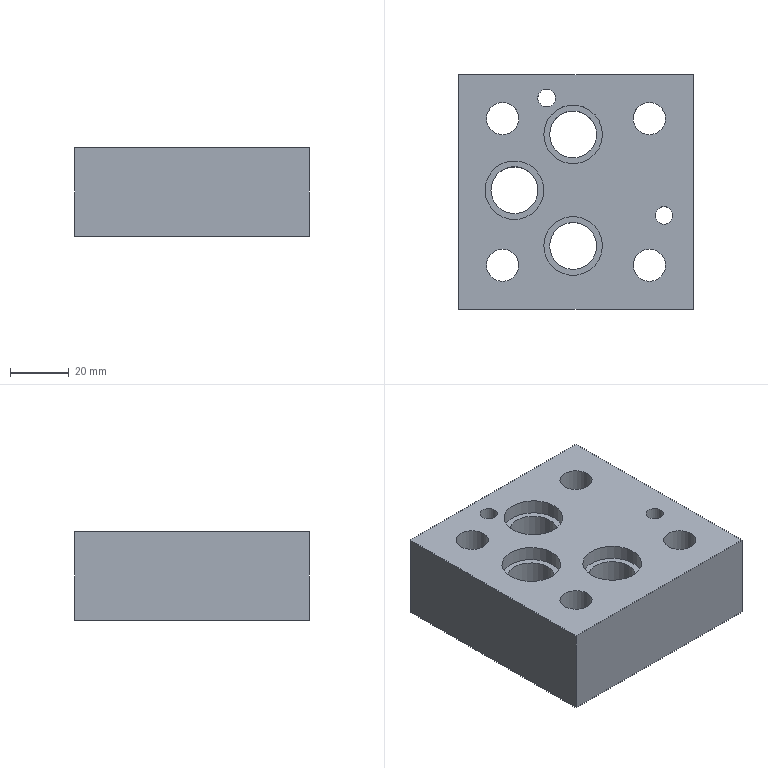Part | NX | features solid 2 | 1 solid | 29 faces | box 80 x 80 x 30 mm | volume 152774 mm3 | cylinder 16 | plane 13 | commonest cylinder face diameters 11 x4 17 x4 16 x3 20 x3 6 x2
STEP:
#1=CARTESIAN_POINT('',(-698.983,-4.404,58.));
#2=VERTEX_POINT('',#1);
#3=CARTESIAN_POINT('',(-690.983,-4.404,58.));
#4=DIRECTION('',(0.,0.,-1.));
#5=DIRECTION('',(-1.,0.,0.));
#6=AXIS2_PLACEMENT_3D('',#3,#4,#5);
#7=CIRCLE('',#6,8.);
#8=EDGE_CURVE('',#2,#2,#7,.F.);
#9=ORIENTED_EDGE('',*,*,#8,.T.);
#10=EDGE_LOOP('',(#9));
#11=FACE_BOUND('',#10,.T.);
#12=CARTESIAN_POINT('',(-703.5,-30.,58.));
#13=VERTEX_POINT('',#12);
#14=CARTESIAN_POINT('',(-695.,-30.,58.));
#15=DIRECTION('',(0.,0.,-1.));
#16=DIRECTION('',(-1.,0.,0.));
#17=AXIS2_PLACEMENT_3D('',#14,#15,#16);
#18=CIRCLE('',#17,8.5);
#19=EDGE_CURVE('',#13,#13,#18,.T.);
#20=ORIENTED_EDGE('',*,*,#19,.F.);
#21=EDGE_LOOP('',(#20));
#22=FACE_BOUND('',#21,.T.);
#23=CARTESIAN_POINT('',(-703.5,20.,58.));
#24=VERTEX_POINT('',#23);
#25=CARTESIAN_POINT('',(-695.,20.,58.));
#26=DIRECTION('',(0.,0.,-1.));
#27=DIRECTION('',(-1.,0.,0.));
#28=AXIS2_PLACEMENT_3D('',#25,#26,#27);
#29=CIRCLE('',#28,8.5);
#30=EDGE_CURVE('',#24,#24,#29,.T.);
#31=ORIENTED_EDGE('',*,*,#30,.F.);
#32=EDGE_LOOP('',(#31));
#33=FACE_BOUND('',#32,.T.);
#34=CARTESIAN_POINT('',(-653.5,20.,58.));
#35=VERTEX_POINT('',#34);
#36=CARTESIAN_POINT('',(-645.,20.,58.));
#37=DIRECTION('',(0.,0.,-1.));
#38=DIRECTION('',(-1.,0.,0.));
#39=AXIS2_PLACEMENT_3D('',#36,#37,#38);
#40=CIRCLE('',#39,8.5);
#41=EDGE_CURVE('',#35,#35,#40,.T.);
#42=ORIENTED_EDGE('',*,*,#41,.F.);
#43=EDGE_LOOP('',(#42));
#44=FACE_BOUND('',#43,.T.);
#45=CARTESIAN_POINT('',(-653.5,-30.,58.));
#46=VERTEX_POINT('',#45);
#47=CARTESIAN_POINT('',(-645.,-30.,58.));
#48=DIRECTION('',(0.,0.,-1.));
#49=DIRECTION('',(-1.,0.,0.));
#50=AXIS2_PLACEMENT_3D('',#47,#48,#49);
#51=CIRCLE('',#50,8.5);
#52=EDGE_CURVE('',#46,#46,#51,.T.);
#53=ORIENTED_EDGE('',*,*,#52,.F.);
#54=EDGE_LOOP('',(#53));
#55=FACE_BOUND('',#54,.T.);
#56=CARTESIAN_POINT('',(-710.,-45.,58.));
#57=VERTEX_POINT('',#56);
#58=CARTESIAN_POINT('',(-710.,35.,58.));
#59=VERTEX_POINT('',#58);
#60=CARTESIAN_POINT('',(-710.,25.,58.));
#61=DIRECTION('',(0.,1.,0.));
#62=VECTOR('',#61,1000.);
#63=LINE('',#60,#62);
#64=EDGE_CURVE('',#57,#59,#63,.T.);
#65=ORIENTED_EDGE('',*,*,#64,.T.);
#66=CARTESIAN_POINT('',(-630.,35.,58.));
#67=VERTEX_POINT('',#66);
#68=CARTESIAN_POINT('',(-720.,35.,58.));
#69=DIRECTION('',(1.,0.,0.));
#70=VECTOR('',#69,1000.);
#71=LINE('',#68,#70);
#72=EDGE_CURVE('',#59,#67,#71,.T.);
#73=ORIENTED_EDGE('',*,*,#72,.T.);
#74=CARTESIAN_POINT('',(-630.,-45.,58.));
#75=VERTEX_POINT('',#74);
#76=CARTESIAN_POINT('',(-630.,25.,58.));
#77=DIRECTION('',(0.,-1.,0.));
#78=VECTOR('',#77,1000.);
#79=LINE('',#76,#78);
#80=EDGE_CURVE('',#67,#75,#79,.T.);
#81=ORIENTED_EDGE('',*,*,#80,.T.);
#82=CARTESIAN_POINT('',(-720.,-45.,58.));
#83=DIRECTION('',(-1.,0.,0.));
#84=VECTOR('',#83,1000.);
#85=LINE('',#82,#84);
#86=EDGE_CURVE('',#75,#57,#85,.T.);
#87=ORIENTED_EDGE('',*,*,#86,.T.);
#88=EDGE_LOOP('',(#65,#73,#81,#87));
#89=FACE_BOUND('',#88,.T.);
#90=CARTESIAN_POINT('',(-678.983,14.595,58.));
#91=VERTEX_POINT('',#90);
#92=CARTESIAN_POINT('',(-670.983,14.595,58.));
#93=DIRECTION('',(0.,0.,-1.));
#94=DIRECTION('',(-1.,0.,0.));
#95=AXIS2_PLACEMENT_3D('',#92,#93,#94);
#96=CIRCLE('',#95,8.);
#97=EDGE_CURVE('',#91,#91,#96,.T.);
#98=ORIENTED_EDGE('',*,*,#97,.F.);
#99=EDGE_LOOP('',(#98));
#100=FACE_BOUND('',#99,.T.);
#101=CARTESIAN_POINT('',(-678.983,-23.404,58.));
#102=VERTEX_POINT('',#101);
#103=CARTESIAN_POINT('',(-670.983,-23.404,58.));
#104=DIRECTION('',(0.,0.,-1.));
#105=DIRECTION('',(-1.,0.,0.));
#106=AXIS2_PLACEMENT_3D('',#103,#104,#105);
#107=CIRCLE('',#106,8.);
#108=EDGE_CURVE('',#102,#102,#107,.F.);
#109=ORIENTED_EDGE('',*,*,#108,.T.);
#110=EDGE_LOOP('',(#109));
#111=FACE_BOUND('',#110,.T.);
#112=CARTESIAN_POINT('',(-637.,-13.,58.));
#113=VERTEX_POINT('',#112);
#114=CARTESIAN_POINT('',(-640.,-13.,58.));
#115=DIRECTION('',(0.,0.,1.));
#116=DIRECTION('',(1.,0.,0.));
#117=AXIS2_PLACEMENT_3D('',#114,#115,#116);
#118=CIRCLE('',#117,3.);
#119=EDGE_CURVE('',#113,#113,#118,.F.);
#120=ORIENTED_EDGE('',*,*,#119,.F.);
#121=EDGE_LOOP('',(#120));
#122=FACE_BOUND('',#121,.T.);
#123=CARTESIAN_POINT('',(-677.,27.,58.));
#124=VERTEX_POINT('',#123);
#125=CARTESIAN_POINT('',(-680.,27.,58.));
#126=DIRECTION('',(0.,0.,1.));
#127=DIRECTION('',(1.,0.,0.));
#128=AXIS2_PLACEMENT_3D('',#125,#126,#127);
#129=CIRCLE('',#128,3.);
#130=EDGE_CURVE('',#124,#124,#129,.F.);
#131=ORIENTED_EDGE('',*,*,#130,.F.);
#132=EDGE_LOOP('',(#131));
#133=FACE_BOUND('',#132,.T.);
#134=CARTESIAN_POINT('',(-720.,25.,58.));
#135=DIRECTION('',(0.,0.,-1.));
#136=DIRECTION('',(1.,0.,0.));
#137=AXIS2_PLACEMENT_3D('',#134,#135,#136);
#138=PLANE('',#137);
#139=ADVANCED_FACE('',(#11,#22,#33,#44,#55,#89,#100,#111,#122,#133),#138,.T.);
#140=ORIENTED_EDGE('',*,*,#97,.T.);
#141=EDGE_LOOP('',(#140));
#142=FACE_BOUND('',#141,.T.);
#143=CARTESIAN_POINT('',(-678.983,14.595,83.));
#144=VERTEX_POINT('',#143);
#145=CARTESIAN_POINT('',(-670.983,14.595,83.));
#146=DIRECTION('',(0.,0.,-1.));
#147=DIRECTION('',(-1.,0.,0.));
#148=AXIS2_PLACEMENT_3D('',#145,#146,#147);
#149=CIRCLE('',#148,8.);
#150=EDGE_CURVE('',#144,#144,#149,.T.);
#151=ORIENTED_EDGE('',*,*,#150,.F.);
#152=EDGE_LOOP('',(#151));
#153=FACE_BOUND('',#152,.T.);
#154=CARTESIAN_POINT('',(-670.983,14.595,88.));
#155=DIRECTION('',(0.,0.,-1.));
#156=DIRECTION('',(1.,0.,0.));
#157=AXIS2_PLACEMENT_3D('',#154,#155,#156);
#158=CYLINDRICAL_SURFACE('',#157,8.);
#159=ADVANCED_FACE('',(#142,#153),#158,.F.);
#160=CARTESIAN_POINT('',(-680.983,-23.404,88.));
#161=VERTEX_POINT('',#160);
#162=CARTESIAN_POINT('',(-670.983,-23.404,88.));
#163=DIRECTION('',(0.,0.,-1.));
#164=DIRECTION('',(-1.,0.,0.));
#165=AXIS2_PLACEMENT_3D('',#162,#163,#164);
#166=CIRCLE('',#165,10.);
#167=EDGE_CURVE('',#161,#161,#166,.T.);
#168=ORIENTED_EDGE('',*,*,#167,.T.);
#169=EDGE_LOOP('',(#168));
#170=FACE_BOUND('',#169,.T.);
#171=CARTESIAN_POINT('',(-700.983,-4.404,88.));
#172=VERTEX_POINT('',#171);
#173=CARTESIAN_POINT('',(-690.983,-4.404,88.));
#174=DIRECTION('',(0.,0.,-1.));
#175=DIRECTION('',(-1.,0.,0.));
#176=AXIS2_PLACEMENT_3D('',#173,#174,#175);
#177=CIRCLE('',#176,10.);
#178=EDGE_CURVE('',#172,#172,#177,.T.);
#179=ORIENTED_EDGE('',*,*,#178,.T.);
#180=EDGE_LOOP('',(#179));
#181=FACE_BOUND('',#180,.T.);
#182=CARTESIAN_POINT('',(-680.983,14.595,88.));
#183=VERTEX_POINT('',#182);
#184=CARTESIAN_POINT('',(-670.983,14.595,88.));
#185=DIRECTION('',(0.,0.,-1.));
#186=DIRECTION('',(-1.,0.,0.));
#187=AXIS2_PLACEMENT_3D('',#184,#185,#186);
#188=CIRCLE('',#187,10.);
#189=EDGE_CURVE('',#183,#183,#188,.T.);
#190=ORIENTED_EDGE('',*,*,#189,.T.);
#191=EDGE_LOOP('',(#190));
#192=FACE_BOUND('',#191,.T.);
#193=CARTESIAN_POINT('',(-700.5,-30.,88.));
#194=VERTEX_POINT('',#193);
#195=CARTESIAN_POINT('',(-695.,-30.,88.));
#196=DIRECTION('',(0.,0.,-1.));
#197=DIRECTION('',(-1.,0.,0.));
#198=AXIS2_PLACEMENT_3D('',#195,#196,#197);
#199=CIRCLE('',#198,5.5);
#200=EDGE_CURVE('',#194,#194,#199,.T.);
#201=ORIENTED_EDGE('',*,*,#200,.T.);
#202=EDGE_LOOP('',(#201));
#203=FACE_BOUND('',#202,.T.);
#204=CARTESIAN_POINT('',(-700.5,20.,88.));
#205=VERTEX_POINT('',#204);
#206=CARTESIAN_POINT('',(-695.,20.,88.));
#207=DIRECTION('',(0.,0.,-1.));
#208=DIRECTION('',(-1.,0.,0.));
#209=AXIS2_PLACEMENT_3D('',#206,#207,#208);
#210=CIRCLE('',#209,5.5);
#211=EDGE_CURVE('',#205,#205,#210,.T.);
#212=ORIENTED_EDGE('',*,*,#211,.T.);
#213=EDGE_LOOP('',(#212));
#214=FACE_BOUND('',#213,.T.);
#215=CARTESIAN_POINT('',(-650.5,20.,88.));
#216=VERTEX_POINT('',#215);
#217=CARTESIAN_POINT('',(-645.,20.,88.));
#218=DIRECTION('',(0.,0.,-1.));
#219=DIRECTION('',(-1.,0.,0.));
#220=AXIS2_PLACEMENT_3D('',#217,#218,#219);
#221=CIRCLE('',#220,5.5);
#222=EDGE_CURVE('',#216,#216,#221,.T.);
#223=ORIENTED_EDGE('',*,*,#222,.T.);
#224=EDGE_LOOP('',(#223));
#225=FACE_BOUND('',#224,.T.);
#226=CARTESIAN_POINT('',(-650.5,-30.,88.));
#227=VERTEX_POINT('',#226);
#228=CARTESIAN_POINT('',(-645.,-30.,88.));
#229=DIRECTION('',(0.,0.,-1.));
#230=DIRECTION('',(-1.,0.,0.));
#231=AXIS2_PLACEMENT_3D('',#228,#229,#230);
#232=CIRCLE('',#231,5.5);
#233=EDGE_CURVE('',#227,#227,#232,.T.);
#234=ORIENTED_EDGE('',*,*,#233,.T.);
#235=EDGE_LOOP('',(#234));
#236=FACE_BOUND('',#235,.T.);
#237=CARTESIAN_POINT('',(-643.,-13.,88.));
#238=VERTEX_POINT('',#237);
#239=CARTESIAN_POINT('',(-640.,-13.,88.));
#240=DIRECTION('',(0.,0.,-1.));
#241=DIRECTION('',(-1.,0.,0.));
#242=AXIS2_PLACEMENT_3D('',#239,#240,#241);
#243=CIRCLE('',#242,3.);
#244=EDGE_CURVE('',#238,#238,#243,.T.);
#245=ORIENTED_EDGE('',*,*,#244,.T.);
#246=EDGE_LOOP('',(#245));
#247=FACE_BOUND('',#246,.T.);
#248=CARTESIAN_POINT('',(-683.,27.,88.));
#249=VERTEX_POINT('',#248);
#250=CARTESIAN_POINT('',(-680.,27.,88.));
#251=DIRECTION('',(0.,0.,-1.));
#252=DIRECTION('',(-1.,0.,0.));
#253=AXIS2_PLACEMENT_3D('',#250,#251,#252);
#254=CIRCLE('',#253,3.);
#255=EDGE_CURVE('',#249,#249,#254,.T.);
#256=ORIENTED_EDGE('',*,*,#255,.T.);
#257=EDGE_LOOP('',(#256));
#258=FACE_BOUND('',#257,.T.);
#259=CARTESIAN_POINT('',(-710.,-45.,88.));
#260=VERTEX_POINT('',#259);
#261=CARTESIAN_POINT('',(-630.,-45.,88.));
#262=VERTEX_POINT('',#261);
#263=CARTESIAN_POINT('',(-720.,-45.,88.));
#264=DIRECTION('',(1.,0.,0.));
#265=VECTOR('',#264,1000.);
#266=LINE('',#263,#265);
#267=EDGE_CURVE('',#260,#262,#266,.T.);
#268=ORIENTED_EDGE('',*,*,#267,.T.);
#269=CARTESIAN_POINT('',(-630.,35.,88.));
#270=VERTEX_POINT('',#269);
#271=CARTESIAN_POINT('',(-630.,25.,88.));
#272=DIRECTION('',(0.,1.,0.));
#273=VECTOR('',#272,1000.);
#274=LINE('',#271,#273);
#275=EDGE_CURVE('',#262,#270,#274,.T.);
#276=ORIENTED_EDGE('',*,*,#275,.T.);
#277=CARTESIAN_POINT('',(-710.,35.,88.));
#278=VERTEX_POINT('',#277);
#279=CARTESIAN_POINT('',(-720.,35.,88.));
#280=DIRECTION('',(-1.,0.,0.));
#281=VECTOR('',#280,1000.);
#282=LINE('',#279,#281);
#283=EDGE_CURVE('',#270,#278,#282,.T.);
#284=ORIENTED_EDGE('',*,*,#283,.T.);
#285=CARTESIAN_POINT('',(-710.,25.,88.));
#286=DIRECTION('',(0.,-1.,0.));
#287=VECTOR('',#286,1000.);
#288=LINE('',#285,#287);
#289=EDGE_CURVE('',#278,#260,#288,.T.);
#290=ORIENTED_EDGE('',*,*,#289,.T.);
#291=EDGE_LOOP('',(#268,#276,#284,#290));
#292=FACE_BOUND('',#291,.T.);
#293=CARTESIAN_POINT('',(-720.,25.,88.));
#294=DIRECTION('',(0.,0.,1.));
#295=DIRECTION('',(-1.,0.,0.));
#296=AXIS2_PLACEMENT_3D('',#293,#294,#295);
#297=PLANE('',#296);
#298=ADVANCED_FACE('',(#170,#181,#192,#203,#214,#225,#236,#247,#258,#292),#297,.T.);
#299=CARTESIAN_POINT('',(-710.,-45.,88.));
#300=DIRECTION('',(0.,0.,1.));
#301=VECTOR('',#300,1000.);
#302=LINE('',#299,#301);
#303=EDGE_CURVE('',#57,#260,#302,.T.);
#304=ORIENTED_EDGE('',*,*,#303,.F.);
#305=ORIENTED_EDGE('',*,*,#86,.F.);
#306=CARTESIAN_POINT('',(-630.,-45.,88.));
#307=DIRECTION('',(0.,0.,1.));
#308=VECTOR('',#307,1000.);
#309=LINE('',#306,#308);
#310=EDGE_CURVE('',#75,#262,#309,.T.);
#311=ORIENTED_EDGE('',*,*,#310,.T.);
#312=ORIENTED_EDGE('',*,*,#267,.F.);
#313=EDGE_LOOP('',(#304,#305,#311,#312));
#314=FACE_BOUND('',#313,.T.);
#315=CARTESIAN_POINT('',(-720.,-45.,88.));
#316=DIRECTION('',(0.,-1.,0.));
#317=DIRECTION('',(0.,0.,-1.));
#318=AXIS2_PLACEMENT_3D('',#315,#316,#317);
#319=PLANE('',#318);
#320=ADVANCED_FACE('',(#314),#319,.T.);
#321=ORIENTED_EDGE('',*,*,#310,.F.);
#322=ORIENTED_EDGE('',*,*,#80,.F.);
#323=CARTESIAN_POINT('',(-630.,35.,88.));
#324=DIRECTION('',(0.,0.,1.));
#325=VECTOR('',#324,1000.);
#326=LINE('',#323,#325);
#327=EDGE_CURVE('',#67,#270,#326,.T.);
#328=ORIENTED_EDGE('',*,*,#327,.T.);
#329=ORIENTED_EDGE('',*,*,#275,.F.);
#330=EDGE_LOOP('',(#321,#322,#328,#329));
#331=FACE_BOUND('',#330,.T.);
#332=CARTESIAN_POINT('',(-630.,25.,88.));
#333=DIRECTION('',(1.,0.,0.));
#334=DIRECTION('',(0.,0.,1.));
#335=AXIS2_PLACEMENT_3D('',#332,#333,#334);
#336=PLANE('',#335);
#337=ADVANCED_FACE('',(#331),#336,.T.);
#338=ORIENTED_EDGE('',*,*,#327,.F.);
#339=ORIENTED_EDGE('',*,*,#72,.F.);
#340=CARTESIAN_POINT('',(-710.,35.,88.));
#341=DIRECTION('',(0.,0.,1.));
#342=VECTOR('',#341,1000.);
#343=LINE('',#340,#342);
#344=EDGE_CURVE('',#59,#278,#343,.T.);
#345=ORIENTED_EDGE('',*,*,#344,.T.);
#346=ORIENTED_EDGE('',*,*,#283,.F.);
#347=EDGE_LOOP('',(#338,#339,#345,#346));
#348=FACE_BOUND('',#347,.T.);
#349=CARTESIAN_POINT('',(-720.,35.,88.));
#350=DIRECTION('',(0.,1.,0.));
#351=DIRECTION('',(0.,0.,1.));
#352=AXIS2_PLACEMENT_3D('',#349,#350,#351);
#353=PLANE('',#352);
#354=ADVANCED_FACE('',(#348),#353,.T.);
#355=ORIENTED_EDGE('',*,*,#64,.F.);
#356=ORIENTED_EDGE('',*,*,#303,.T.);
#357=ORIENTED_EDGE('',*,*,#289,.F.);
#358=ORIENTED_EDGE('',*,*,#344,.F.);
#359=EDGE_LOOP('',(#355,#356,#357,#358));
#360=FACE_BOUND('',#359,.T.);
#361=CARTESIAN_POINT('',(-710.,25.,88.));
#362=DIRECTION('',(-1.,0.,0.));
#363=DIRECTION('',(0.,0.,-1.));
#364=AXIS2_PLACEMENT_3D('',#361,#362,#363);
#365=PLANE('',#364);
#366=ADVANCED_FACE('',(#360),#365,.T.);
#367=ORIENTED_EDGE('',*,*,#255,.F.);
#368=EDGE_LOOP('',(#367));
#369=FACE_BOUND('',#368,.T.);
#370=ORIENTED_EDGE('',*,*,#130,.T.);
#371=EDGE_LOOP('',(#370));
#372=FACE_BOUND('',#371,.T.);
#373=CARTESIAN_POINT('',(-680.,27.,108.));
#374=DIRECTION('',(0.,0.,1.));
#375=DIRECTION('',(-1.,0.,0.));
#376=AXIS2_PLACEMENT_3D('',#373,#374,#375);
#377=CYLINDRICAL_SURFACE('',#376,3.);
#378=ADVANCED_FACE('',(#369,#372),#377,.F.);
#379=ORIENTED_EDGE('',*,*,#244,.F.);
#380=EDGE_LOOP('',(#379));
#381=FACE_BOUND('',#380,.T.);
#382=ORIENTED_EDGE('',*,*,#119,.T.);
#383=EDGE_LOOP('',(#382));
#384=FACE_BOUND('',#383,.T.);
#385=CARTESIAN_POINT('',(-640.,-13.,108.));
#386=DIRECTION('',(0.,0.,1.));
#387=DIRECTION('',(-1.,0.,0.));
#388=AXIS2_PLACEMENT_3D('',#385,#386,#387);
#389=CYLINDRICAL_SURFACE('',#388,3.);
#390=ADVANCED_FACE('',(#381,#384),#389,.F.);
#391=ORIENTED_EDGE('',*,*,#233,.F.);
#392=EDGE_LOOP('',(#391));
#393=FACE_BOUND('',#392,.T.);
#394=CARTESIAN_POINT('',(-650.5,-30.,70.));
#395=VERTEX_POINT('',#394);
#396=CARTESIAN_POINT('',(-645.,-30.,70.));
#397=DIRECTION('',(0.,0.,-1.));
#398=DIRECTION('',(-1.,0.,0.));
#399=AXIS2_PLACEMENT_3D('',#396,#397,#398);
#400=CIRCLE('',#399,5.5);
#401=EDGE_CURVE('',#395,#395,#400,.T.);
#402=ORIENTED_EDGE('',*,*,#401,.T.);
#403=EDGE_LOOP('',(#402));
#404=FACE_BOUND('',#403,.T.);
#405=CARTESIAN_POINT('',(-645.,-30.,108.));
#406=DIRECTION('',(0.,0.,1.));
#407=DIRECTION('',(-1.,0.,0.));
#408=AXIS2_PLACEMENT_3D('',#405,#406,#407);
#409=CYLINDRICAL_SURFACE('',#408,5.5);
#410=ADVANCED_FACE('',(#393,#404),#409,.F.);
#411=ORIENTED_EDGE('',*,*,#401,.F.);
#412=EDGE_LOOP('',(#411));
#413=FACE_BOUND('',#412,.T.);
#414=CARTESIAN_POINT('',(-653.5,-30.,70.));
#415=VERTEX_POINT('',#414);
#416=CARTESIAN_POINT('',(-645.,-30.,70.));
#417=DIRECTION('',(0.,0.,-1.));
#418=DIRECTION('',(-1.,0.,0.));
#419=AXIS2_PLACEMENT_3D('',#416,#417,#418);
#420=CIRCLE('',#419,8.5);
#421=EDGE_CURVE('',#415,#415,#420,.T.);
#422=ORIENTED_EDGE('',*,*,#421,.T.);
#423=EDGE_LOOP('',(#422));
#424=FACE_BOUND('',#423,.T.);
#425=CARTESIAN_POINT('',(-645.,-30.,70.));
#426=DIRECTION('',(0.,0.,1.));
#427=DIRECTION('',(-1.,0.,0.));
#428=AXIS2_PLACEMENT_3D('',#425,#426,#427);
#429=PLANE('',#428);
#430=ADVANCED_FACE('',(#413,#424),#429,.F.);
#431=ORIENTED_EDGE('',*,*,#421,.F.);
#432=EDGE_LOOP('',(#431));
#433=FACE_BOUND('',#432,.T.);
#434=ORIENTED_EDGE('',*,*,#52,.T.);
#435=EDGE_LOOP('',(#434));
#436=FACE_BOUND('',#435,.T.);
#437=CARTESIAN_POINT('',(-645.,-30.,58.));
#438=DIRECTION('',(0.,0.,1.));
#439=DIRECTION('',(-1.,0.,0.));
#440=AXIS2_PLACEMENT_3D('',#437,#438,#439);
#441=CYLINDRICAL_SURFACE('',#440,8.5);
#442=ADVANCED_FACE('',(#433,#436),#441,.F.);
#443=ORIENTED_EDGE('',*,*,#222,.F.);
#444=EDGE_LOOP('',(#443));
#445=FACE_BOUND('',#444,.T.);
#446=CARTESIAN_POINT('',(-650.5,20.,70.));
#447=VERTEX_POINT('',#446);
#448=CARTESIAN_POINT('',(-645.,20.,70.));
#449=DIRECTION('',(0.,0.,-1.));
#450=DIRECTION('',(-1.,0.,0.));
#451=AXIS2_PLACEMENT_3D('',#448,#449,#450);
#452=CIRCLE('',#451,5.5);
#453=EDGE_CURVE('',#447,#447,#452,.T.);
#454=ORIENTED_EDGE('',*,*,#453,.T.);
#455=EDGE_LOOP('',(#454));
#456=FACE_BOUND('',#455,.T.);
#457=CARTESIAN_POINT('',(-645.,20.,108.));
#458=DIRECTION('',(0.,0.,1.));
#459=DIRECTION('',(-1.,0.,0.));
#460=AXIS2_PLACEMENT_3D('',#457,#458,#459);
#461=CYLINDRICAL_SURFACE('',#460,5.5);
#462=ADVANCED_FACE('',(#445,#456),#461,.F.);
#463=ORIENTED_EDGE('',*,*,#453,.F.);
#464=EDGE_LOOP('',(#463));
#465=FACE_BOUND('',#464,.T.);
#466=CARTESIAN_POINT('',(-653.5,20.,70.));
#467=VERTEX_POINT('',#466);
#468=CARTESIAN_POINT('',(-645.,20.,70.));
#469=DIRECTION('',(0.,0.,-1.));
#470=DIRECTION('',(-1.,0.,0.));
#471=AXIS2_PLACEMENT_3D('',#468,#469,#470);
#472=CIRCLE('',#471,8.5);
#473=EDGE_CURVE('',#467,#467,#472,.T.);
#474=ORIENTED_EDGE('',*,*,#473,.T.);
#475=EDGE_LOOP('',(#474));
#476=FACE_BOUND('',#475,.T.);
#477=CARTESIAN_POINT('',(-645.,20.,70.));
#478=DIRECTION('',(0.,0.,1.));
#479=DIRECTION('',(-1.,0.,0.));
#480=AXIS2_PLACEMENT_3D('',#477,#478,#479);
#481=PLANE('',#480);
#482=ADVANCED_FACE('',(#465,#476),#481,.F.);
#483=ORIENTED_EDGE('',*,*,#473,.F.);
#484=EDGE_LOOP('',(#483));
#485=FACE_BOUND('',#484,.T.);
#486=ORIENTED_EDGE('',*,*,#41,.T.);
#487=EDGE_LOOP('',(#486));
#488=FACE_BOUND('',#487,.T.);
#489=CARTESIAN_POINT('',(-645.,20.,58.));
#490=DIRECTION('',(0.,0.,1.));
#491=DIRECTION('',(-1.,0.,0.));
#492=AXIS2_PLACEMENT_3D('',#489,#490,#491);
#493=CYLINDRICAL_SURFACE('',#492,8.5);
#494=ADVANCED_FACE('',(#485,#488),#493,.F.);
#495=ORIENTED_EDGE('',*,*,#211,.F.);
#496=EDGE_LOOP('',(#495));
#497=FACE_BOUND('',#496,.T.);
#498=CARTESIAN_POINT('',(-700.5,20.,70.));
#499=VERTEX_POINT('',#498);
#500=CARTESIAN_POINT('',(-695.,20.,70.));
#501=DIRECTION('',(0.,0.,-1.));
#502=DIRECTION('',(-1.,0.,0.));
#503=AXIS2_PLACEMENT_3D('',#500,#501,#502);
#504=CIRCLE('',#503,5.5);
#505=EDGE_CURVE('',#499,#499,#504,.T.);
#506=ORIENTED_EDGE('',*,*,#505,.T.);
#507=EDGE_LOOP('',(#506));
#508=FACE_BOUND('',#507,.T.);
#509=CARTESIAN_POINT('',(-695.,20.,108.));
#510=DIRECTION('',(0.,0.,1.));
#511=DIRECTION('',(-1.,0.,0.));
#512=AXIS2_PLACEMENT_3D('',#509,#510,#511);
#513=CYLINDRICAL_SURFACE('',#512,5.5);
#514=ADVANCED_FACE('',(#497,#508),#513,.F.);
#515=ORIENTED_EDGE('',*,*,#505,.F.);
#516=EDGE_LOOP('',(#515));
#517=FACE_BOUND('',#516,.T.);
#518=CARTESIAN_POINT('',(-703.5,20.,70.));
#519=VERTEX_POINT('',#518);
#520=CARTESIAN_POINT('',(-695.,20.,70.));
#521=DIRECTION('',(0.,0.,-1.));
#522=DIRECTION('',(-1.,0.,0.));
#523=AXIS2_PLACEMENT_3D('',#520,#521,#522);
#524=CIRCLE('',#523,8.5);
#525=EDGE_CURVE('',#519,#519,#524,.T.);
#526=ORIENTED_EDGE('',*,*,#525,.T.);
#527=EDGE_LOOP('',(#526));
#528=FACE_BOUND('',#527,.T.);
#529=CARTESIAN_POINT('',(-695.,20.,70.));
#530=DIRECTION('',(0.,0.,1.));
#531=DIRECTION('',(-1.,0.,0.));
#532=AXIS2_PLACEMENT_3D('',#529,#530,#531);
#533=PLANE('',#532);
#534=ADVANCED_FACE('',(#517,#528),#533,.F.);
#535=ORIENTED_EDGE('',*,*,#525,.F.);
#536=EDGE_LOOP('',(#535));
#537=FACE_BOUND('',#536,.T.);
#538=ORIENTED_EDGE('',*,*,#30,.T.);
#539=EDGE_LOOP('',(#538));
#540=FACE_BOUND('',#539,.T.);
#541=CARTESIAN_POINT('',(-695.,20.,58.));
#542=DIRECTION('',(0.,0.,1.));
#543=DIRECTION('',(-1.,0.,0.));
#544=AXIS2_PLACEMENT_3D('',#541,#542,#543);
#545=CYLINDRICAL_SURFACE('',#544,8.5);
#546=ADVANCED_FACE('',(#537,#540),#545,.F.);
#547=ORIENTED_EDGE('',*,*,#200,.F.);
#548=EDGE_LOOP('',(#547));
#549=FACE_BOUND('',#548,.T.);
#550=CARTESIAN_POINT('',(-700.5,-30.,70.));
#551=VERTEX_POINT('',#550);
#552=CARTESIAN_POINT('',(-695.,-30.,70.));
#553=DIRECTION('',(0.,0.,-1.));
#554=DIRECTION('',(-1.,0.,0.));
#555=AXIS2_PLACEMENT_3D('',#552,#553,#554);
#556=CIRCLE('',#555,5.5);
#557=EDGE_CURVE('',#551,#551,#556,.T.);
#558=ORIENTED_EDGE('',*,*,#557,.T.);
#559=EDGE_LOOP('',(#558));
#560=FACE_BOUND('',#559,.T.);
#561=CARTESIAN_POINT('',(-695.,-30.,108.));
#562=DIRECTION('',(0.,0.,1.));
#563=DIRECTION('',(-1.,0.,0.));
#564=AXIS2_PLACEMENT_3D('',#561,#562,#563);
#565=CYLINDRICAL_SURFACE('',#564,5.5);
#566=ADVANCED_FACE('',(#549,#560),#565,.F.);
#567=ORIENTED_EDGE('',*,*,#557,.F.);
#568=EDGE_LOOP('',(#567));
#569=FACE_BOUND('',#568,.T.);
#570=CARTESIAN_POINT('',(-703.5,-30.,70.));
#571=VERTEX_POINT('',#570);
#572=CARTESIAN_POINT('',(-695.,-30.,70.));
#573=DIRECTION('',(0.,0.,-1.));
#574=DIRECTION('',(-1.,0.,0.));
#575=AXIS2_PLACEMENT_3D('',#572,#573,#574);
#576=CIRCLE('',#575,8.5);
#577=EDGE_CURVE('',#571,#571,#576,.T.);
#578=ORIENTED_EDGE('',*,*,#577,.T.);
#579=EDGE_LOOP('',(#578));
#580=FACE_BOUND('',#579,.T.);
#581=CARTESIAN_POINT('',(-695.,-30.,70.));
#582=DIRECTION('',(0.,0.,1.));
#583=DIRECTION('',(-1.,0.,0.));
#584=AXIS2_PLACEMENT_3D('',#581,#582,#583);
#585=PLANE('',#584);
#586=ADVANCED_FACE('',(#569,#580),#585,.F.);
#587=ORIENTED_EDGE('',*,*,#577,.F.);
#588=EDGE_LOOP('',(#587));
#589=FACE_BOUND('',#588,.T.);
#590=ORIENTED_EDGE('',*,*,#19,.T.);
#591=EDGE_LOOP('',(#590));
#592=FACE_BOUND('',#591,.T.);
#593=CARTESIAN_POINT('',(-695.,-30.,58.));
#594=DIRECTION('',(0.,0.,1.));
#595=DIRECTION('',(-1.,0.,0.));
#596=AXIS2_PLACEMENT_3D('',#593,#594,#595);
#597=CYLINDRICAL_SURFACE('',#596,8.5);
#598=ADVANCED_FACE('',(#589,#592),#597,.F.);
#599=CARTESIAN_POINT('',(-680.983,14.595,83.));
#600=VERTEX_POINT('',#599);
#601=CARTESIAN_POINT('',(-670.983,14.595,83.));
#602=DIRECTION('',(0.,0.,-1.));
#603=DIRECTION('',(-1.,0.,0.));
#604=AXIS2_PLACEMENT_3D('',#601,#602,#603);
#605=CIRCLE('',#604,10.);
#606=EDGE_CURVE('',#600,#600,#605,.T.);
#607=ORIENTED_EDGE('',*,*,#606,.F.);
#608=EDGE_LOOP('',(#607));
#609=FACE_BOUND('',#608,.T.);
#610=ORIENTED_EDGE('',*,*,#150,.T.);
#611=EDGE_LOOP('',(#610));
#612=FACE_BOUND('',#611,.T.);
#613=CARTESIAN_POINT('',(-670.983,14.595,83.));
#614=DIRECTION('',(0.,0.,1.));
#615=DIRECTION('',(-1.,0.,0.));
#616=AXIS2_PLACEMENT_3D('',#613,#614,#615);
#617=PLANE('',#616);
#618=ADVANCED_FACE('',(#609,#612),#617,.T.);
#619=ORIENTED_EDGE('',*,*,#606,.T.);
#620=EDGE_LOOP('',(#619));
#621=FACE_BOUND('',#620,.T.);
#622=ORIENTED_EDGE('',*,*,#189,.F.);
#623=EDGE_LOOP('',(#622));
#624=FACE_BOUND('',#623,.T.);
#625=CARTESIAN_POINT('',(-670.983,14.595,83.));
#626=DIRECTION('',(0.,0.,1.));
#627=DIRECTION('',(-1.,0.,0.));
#628=AXIS2_PLACEMENT_3D('',#625,#626,#627);
#629=CYLINDRICAL_SURFACE('',#628,10.);
#630=ADVANCED_FACE('',(#621,#624),#629,.F.);
#631=ORIENTED_EDGE('',*,*,#8,.F.);
#632=EDGE_LOOP('',(#631));
#633=FACE_BOUND('',#632,.T.);
#634=CARTESIAN_POINT('',(-698.983,-4.404,83.));
#635=VERTEX_POINT('',#634);
#636=CARTESIAN_POINT('',(-690.983,-4.404,83.));
#637=DIRECTION('',(0.,0.,-1.));
#638=DIRECTION('',(-1.,0.,0.));
#639=AXIS2_PLACEMENT_3D('',#636,#637,#638);
#640=CIRCLE('',#639,8.);
#641=EDGE_CURVE('',#635,#635,#640,.T.);
#642=ORIENTED_EDGE('',*,*,#641,.F.);
#643=EDGE_LOOP('',(#642));
#644=FACE_BOUND('',#643,.T.);
#645=CARTESIAN_POINT('',(-690.983,-4.404,88.));
#646=DIRECTION('',(0.,0.,-1.));
#647=DIRECTION('',(1.,0.,0.));
#648=AXIS2_PLACEMENT_3D('',#645,#646,#647);
#649=CYLINDRICAL_SURFACE('',#648,8.);
#650=ADVANCED_FACE('',(#633,#644),#649,.F.);
#651=CARTESIAN_POINT('',(-700.983,-4.404,83.));
#652=VERTEX_POINT('',#651);
#653=CARTESIAN_POINT('',(-690.983,-4.404,83.));
#654=DIRECTION('',(0.,0.,-1.));
#655=DIRECTION('',(-1.,0.,0.));
#656=AXIS2_PLACEMENT_3D('',#653,#654,#655);
#657=CIRCLE('',#656,10.);
#658=EDGE_CURVE('',#652,#652,#657,.T.);
#659=ORIENTED_EDGE('',*,*,#658,.F.);
#660=EDGE_LOOP('',(#659));
#661=FACE_BOUND('',#660,.T.);
#662=ORIENTED_EDGE('',*,*,#641,.T.);
#663=EDGE_LOOP('',(#662));
#664=FACE_BOUND('',#663,.T.);
#665=CARTESIAN_POINT('',(-690.983,-4.404,83.));
#666=DIRECTION('',(0.,0.,1.));
#667=DIRECTION('',(-1.,0.,0.));
#668=AXIS2_PLACEMENT_3D('',#665,#666,#667);
#669=PLANE('',#668);
#670=ADVANCED_FACE('',(#661,#664),#669,.T.);
#671=ORIENTED_EDGE('',*,*,#658,.T.);
#672=EDGE_LOOP('',(#671));
#673=FACE_BOUND('',#672,.T.);
#674=ORIENTED_EDGE('',*,*,#178,.F.);
#675=EDGE_LOOP('',(#674));
#676=FACE_BOUND('',#675,.T.);
#677=CARTESIAN_POINT('',(-690.983,-4.404,83.));
#678=DIRECTION('',(0.,0.,1.));
#679=DIRECTION('',(-1.,0.,0.));
#680=AXIS2_PLACEMENT_3D('',#677,#678,#679);
#681=CYLINDRICAL_SURFACE('',#680,10.);
#682=ADVANCED_FACE('',(#673,#676),#681,.F.);
#683=ORIENTED_EDGE('',*,*,#108,.F.);
#684=EDGE_LOOP('',(#683));
#685=FACE_BOUND('',#684,.T.);
#686=CARTESIAN_POINT('',(-678.983,-23.404,83.));
#687=VERTEX_POINT('',#686);
#688=CARTESIAN_POINT('',(-670.983,-23.404,83.));
#689=DIRECTION('',(0.,0.,-1.));
#690=DIRECTION('',(-1.,0.,0.));
#691=AXIS2_PLACEMENT_3D('',#688,#689,#690);
#692=CIRCLE('',#691,8.);
#693=EDGE_CURVE('',#687,#687,#692,.T.);
#694=ORIENTED_EDGE('',*,*,#693,.F.);
#695=EDGE_LOOP('',(#694));
#696=FACE_BOUND('',#695,.T.);
#697=CARTESIAN_POINT('',(-670.983,-23.404,88.));
#698=DIRECTION('',(0.,0.,-1.));
#699=DIRECTION('',(1.,0.,0.));
#700=AXIS2_PLACEMENT_3D('',#697,#698,#699);
#701=CYLINDRICAL_SURFACE('',#700,8.);
#702=ADVANCED_FACE('',(#685,#696),#701,.F.);
#703=CARTESIAN_POINT('',(-680.983,-23.404,83.));
#704=VERTEX_POINT('',#703);
#705=CARTESIAN_POINT('',(-670.983,-23.404,83.));
#706=DIRECTION('',(0.,0.,-1.));
#707=DIRECTION('',(-1.,0.,0.));
#708=AXIS2_PLACEMENT_3D('',#705,#706,#707);
#709=CIRCLE('',#708,10.);
#710=EDGE_CURVE('',#704,#704,#709,.T.);
#711=ORIENTED_EDGE('',*,*,#710,.F.);
#712=EDGE_LOOP('',(#711));
#713=FACE_BOUND('',#712,.T.);
#714=ORIENTED_EDGE('',*,*,#693,.T.);
#715=EDGE_LOOP('',(#714));
#716=FACE_BOUND('',#715,.T.);
#717=CARTESIAN_POINT('',(-670.983,-23.404,83.));
#718=DIRECTION('',(0.,0.,1.));
#719=DIRECTION('',(-1.,0.,0.));
#720=AXIS2_PLACEMENT_3D('',#717,#718,#719);
#721=PLANE('',#720);
#722=ADVANCED_FACE('',(#713,#716),#721,.T.);
#723=ORIENTED_EDGE('',*,*,#710,.T.);
#724=EDGE_LOOP('',(#723));
#725=FACE_BOUND('',#724,.T.);
#726=ORIENTED_EDGE('',*,*,#167,.F.);
#727=EDGE_LOOP('',(#726));
#728=FACE_BOUND('',#727,.T.);
#729=CARTESIAN_POINT('',(-670.983,-23.404,83.));
#730=DIRECTION('',(0.,0.,1.));
#731=DIRECTION('',(-1.,0.,0.));
#732=AXIS2_PLACEMENT_3D('',#729,#730,#731);
#733=CYLINDRICAL_SURFACE('',#732,10.);
#734=ADVANCED_FACE('',(#725,#728),#733,.F.);
#735=CLOSED_SHELL('',(#139,#159,#298,#320,#337,#354,#366,#378,#390,#410,#430,#442,#462,#482,#494,#514,#534,#546,#566,#586,#598,#618,#630,#650,#670,#682,#702,#722,#734));
#736=MANIFOLD_SOLID_BREP('',#735);
#737=(LENGTH_UNIT()NAMED_UNIT(*)SI_UNIT(.MILLI.,.METRE.));
#738=UNCERTAINTY_MEASURE_WITH_UNIT(LENGTH_MEASURE(0.00001),#737,'','');
#739=(NAMED_UNIT(*)PLANE_ANGLE_UNIT()SI_UNIT($,.RADIAN.));
#740=(NAMED_UNIT(*)SI_UNIT($,.STERADIAN.)SOLID_ANGLE_UNIT());
#741=(GEOMETRIC_REPRESENTATION_CONTEXT(3)GLOBAL_UNCERTAINTY_ASSIGNED_CONTEXT((#738))GLOBAL_UNIT_ASSIGNED_CONTEXT((#737,#739,#740))REPRESENTATION_CONTEXT('',''));
#742=ADVANCED_BREP_SHAPE_REPRESENTATION('',(#736),#741);